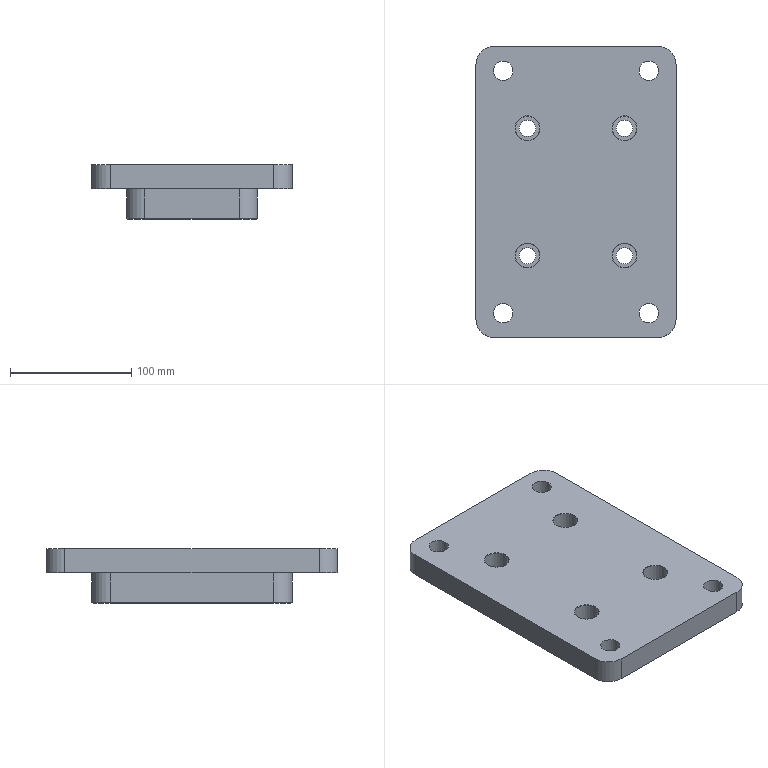NC program | NX | posted with a generic post | part box 165 x 240 x 45 mm
Lines 1 to 2077 of 2364, first 1783 of 2069 lines:
N10 G17 G21 G94 G90
(ZLEVEL_PROFILE_COPY , TOOL : D25R0.5)
N12 T05 M6
N14 G54
N16 G17 G0 G90 X-124.057 Y-0.073 S2000 M3
N18 G43 Z30. H5
N20 Z3.
N22 G94 G1 Y40.842 Z1.929 F1000.
N24 X-123.672 Y45.838 Z1.797
N26 X-122.847 Y50.78 Z1.666
N28 X-121.589 Y55.629 Z1.535
N30 X-119.906 Y60.348 Z1.404
N32 X-117.812 Y64.9 Z1.273
N34 X-115.324 Y69.249 Z1.141
N36 X-112.461 Y73.36 Z1.01
N38 X-109.245 Y77.203 Z0.879
N40 X-105.703 Y80.745 Z0.748
N42 X-101.86 Y83.961 Z0.617
N44 X-97.749 Y86.824 Z0.485
N46 X-93.4 Y89.312 Z0.354
N48 X-88.848 Y91.406 Z0.223
N50 X-84.129 Y93.089 Z0.092
N52 X-79.28 Y94.347 Z-0.039
N54 X-74.338 Y95.172 Z-0.171
N56 X-69.342 Y95.557 Z-0.302
N58 X-67.5 Z-0.35
N60 X67.5 F2200.
N62 G2 X124.057 Y39. R56.557
N64 G1 Y-39.
N66 G2 X67.5 Y-95.557 R56.557
N68 G1 X-67.5
N70 G2 X-124.057 Y-39. R56.557
N72 G1 Y39.
N74 G2 X-67.5 Y95.557 R56.557
N76 G1 X-47.449 Y95.907 Z-0.7
N78 X67.5
N80 G2 X124.407 Y39. R56.907
N82 G1 Y-39.
N84 G2 X67.5 Y-95.907 R56.907
N86 G1 X-67.5
N88 G2 X-124.407 Y-39. R56.907
N90 G1 Y39.
N92 G2 X-67.5 Y95.907 R56.907
N94 G1 X-47.449 Y96.257 Z-1.05
N96 X67.5
N98 G2 X124.757 Y39. R57.257
N100 G1 Y-39.
N102 G2 X67.5 Y-96.257 R57.257
N104 G1 X-67.5
N106 G2 X-124.757 Y-39. R57.257
N108 G1 Y39.
N110 G2 X-67.5 Y96.257 R57.257
N112 G1 X-63.044 Y96.335 Z-1.128
N114 X-61.93 Y96.354 Z-1.147
N116 X-60.816 Y96.373 Z-1.167
N118 X-59.702 Y96.389 Z-1.186
N120 X-58.588 Y96.404 Z-1.206
N122 X-57.474 Y96.418 Z-1.225
N124 X-56.36 Y96.43 Z-1.244
N126 X-55.246 Y96.441 Z-1.264
N128 X-54.132 Y96.451 Z-1.283
N130 X-53.018 Y96.459 Z-1.303
N132 X-51.904 Y96.467 Z-1.322
N134 X-50.79 Y96.474 Z-1.342
N136 X-49.676 Y96.48 Z-1.361
N138 X-48.562 Y96.486 Z-1.381
N140 X-47.449 Y96.49 Z-1.4
N142 X67.5
N144 G2 X124.99 Y39. R57.49
N146 G1 Y-39.
N148 G2 X67.5 Y-96.49 R57.49
N150 G1 X-67.5
N152 G2 X-124.99 Y-39. R57.49
N154 G1 Y39.
N156 G2 X-67.5 Y96.49 R57.49
N158 G1 X-66.386 Y96.493 Z-1.419
N160 X-65.272 Y96.496 Z-1.439
N162 X-64.158 Y96.498 Z-1.458
N164 X-63.044 Y96.5 Z-1.478
N166 X-61.93 Z-1.497
N168 X-60.816 Z-1.517
N170 X-47.449 Z-1.75
N172 X67.5
N174 G2 X125. Y39. R57.5
N176 G1 Y-39.
N178 G2 X67.5 Y-96.5 R57.5
N180 G1 X-67.5
N182 G2 X-125. Y-39. R57.5
N184 G1 Y39.
N186 G2 X-67.5 Y96.5 R57.5
N188 G1 X-47.449 Z-2.1
N190 X67.5
N192 G2 X125. Y39. R57.5
N194 G1 Y-39.
N196 G2 X67.5 Y-96.5 R57.5
N198 G1 X-67.5
N200 G2 X-125. Y-39. R57.5
N202 G1 Y39.
N204 G2 X-67.5 Y96.5 R57.5
N206 G1 X-47.449 Z-2.45
N208 X67.5
N210 G2 X125. Y39. R57.5
N212 G1 Y-39.
N214 G2 X67.5 Y-96.5 R57.5
N216 G1 X-67.5
N218 G2 X-125. Y-39. R57.5
N220 G1 Y39.
N222 G2 X-67.5 Y96.5 R57.5
N224 G1 X-47.449 Z-2.8
N226 X67.5
N228 G2 X125. Y39. R57.5
N230 G1 Y-39.
N232 G2 X67.5 Y-96.5 R57.5
N234 G1 X-67.5
N236 G2 X-125. Y-39. R57.5
N238 G1 Y39.
N240 G2 X-67.5 Y96.5 R57.5
N242 G1 X-47.449 Z-3.15
N244 X67.5
N246 G2 X125. Y39. R57.5
N248 G1 Y-39.
N250 G2 X67.5 Y-96.5 R57.5
N252 G1 X-67.5
N254 G2 X-125. Y-39. R57.5
N256 G1 Y39.
N258 G2 X-67.5 Y96.5 R57.5
N260 G1 X-47.449 Z-3.5
N262 X67.5
N264 G2 X125. Y39. R57.5
N266 G1 Y-39.
N268 G2 X67.5 Y-96.5 R57.5
N270 G1 X-67.5
N272 G2 X-125. Y-39. R57.5
N274 G1 Y39.
N276 G2 X-67.5 Y96.5 R57.5
N278 G1 X-47.449 Z-3.85
N280 X67.5
N282 G2 X125. Y39. R57.5
N284 G1 Y-39.
N286 G2 X67.5 Y-96.5 R57.5
N288 G1 X-67.5
N290 G2 X-125. Y-39. R57.5
N292 G1 Y39.
N294 G2 X-67.5 Y96.5 R57.5
N296 G1 X-47.449 Z-4.2
N298 X67.5
N300 G2 X125. Y39. R57.5
N302 G1 Y-39.
N304 G2 X67.5 Y-96.5 R57.5
N306 G1 X-67.5
N308 G2 X-125. Y-39. R57.5
N310 G1 Y39.
N312 G2 X-67.5 Y96.5 R57.5
N314 G1 X-47.449 Z-4.55
N316 X67.5
N318 G2 X125. Y39. R57.5
N320 G1 Y-39.
N322 G2 X67.5 Y-96.5 R57.5
N324 G1 X-67.5
N326 G2 X-125. Y-39. R57.5
N328 G1 Y39.
N330 G2 X-67.5 Y96.5 R57.5
N332 G1 X-47.449 Z-4.9
N334 X67.5
N336 G2 X125. Y39. R57.5
N338 G1 Y-39.
N340 G2 X67.5 Y-96.5 R57.5
N342 G1 X-67.5
N344 G2 X-125. Y-39. R57.5
N346 G1 Y39.
N348 G2 X-67.5 Y96.5 R57.5
N350 G1 X-47.449 Z-5.25
N352 X67.5
N354 G2 X125. Y39. R57.5
N356 G1 Y-39.
N358 G2 X67.5 Y-96.5 R57.5
N360 G1 X-67.5
N362 G2 X-125. Y-39. R57.5
N364 G1 Y39.
N366 G2 X-67.5 Y96.5 R57.5
N368 G1 X-47.449 Z-5.6
N370 X67.5
N372 G2 X125. Y39. R57.5
N374 G1 Y-39.
N376 G2 X67.5 Y-96.5 R57.5
N378 G1 X-67.5
N380 G2 X-125. Y-39. R57.5
N382 G1 Y39.
N384 G2 X-67.5 Y96.5 R57.5
N386 G1 X-47.449 Z-5.95
N388 X67.5
N390 G2 X125. Y39. R57.5
N392 G1 Y-39.
N394 G2 X67.5 Y-96.5 R57.5
N396 G1 X-67.5
N398 G2 X-125. Y-39. R57.5
N400 G1 Y39.
N402 G2 X-67.5 Y96.5 R57.5
N404 G1 X-47.449 Z-6.3
N406 X67.5
N408 G2 X125. Y39. R57.5
N410 G1 Y-39.
N412 G2 X67.5 Y-96.5 R57.5
N414 G1 X-67.5
N416 G2 X-125. Y-39. R57.5
N418 G1 Y39.
N420 G2 X-67.5 Y96.5 R57.5
N422 G1 X-47.449 Z-6.65
N424 X67.5
N426 G2 X125. Y39. R57.5
N428 G1 Y-39.
N430 G2 X67.5 Y-96.5 R57.5
N432 G1 X-67.5
N434 G2 X-125. Y-39. R57.5
N436 G1 Y39.
N438 G2 X-67.5 Y96.5 R57.5
N440 G1 X-47.449 Z-7.
N442 X67.5
N444 G2 X125. Y39. R57.5
N446 G1 Y-39.
N448 G2 X67.5 Y-96.5 R57.5
N450 G1 X-67.5
N452 G2 X-125. Y-39. R57.5
N454 G1 Y39.
N456 G2 X-67.5 Y96.5 R57.5
N458 G1 X-47.449 Z-7.35
N460 X67.5
N462 G2 X125. Y39. R57.5
N464 G1 Y-39.
N466 G2 X67.5 Y-96.5 R57.5
N468 G1 X-67.5
N470 G2 X-125. Y-39. R57.5
N472 G1 Y39.
N474 G2 X-67.5 Y96.5 R57.5
N476 G1 X-47.449 Z-7.7
N478 X67.5
N480 G2 X125. Y39. R57.5
N482 G1 Y-39.
N484 G2 X67.5 Y-96.5 R57.5
N486 G1 X-67.5
N488 G2 X-125. Y-39. R57.5
N490 G1 Y39.
N492 G2 X-67.5 Y96.5 R57.5
N494 G1 X-47.449 Z-8.05
N496 X67.5
N498 G2 X125. Y39. R57.5
N500 G1 Y-39.
N502 G2 X67.5 Y-96.5 R57.5
N504 G1 X-67.5
N506 G2 X-125. Y-39. R57.5
N508 G1 Y39.
N510 G2 X-67.5 Y96.5 R57.5
N512 G1 X-47.449 Z-8.4
N514 X67.5
N516 G2 X125. Y39. R57.5
N518 G1 Y-39.
N520 G2 X67.5 Y-96.5 R57.5
N522 G1 X-67.5
N524 G2 X-125. Y-39. R57.5
N526 G1 Y39.
N528 G2 X-67.5 Y96.5 R57.5
N530 G1 X-47.449 Z-8.75
N532 X67.5
N534 G2 X125. Y39. R57.5
N536 G1 Y-39.
N538 G2 X67.5 Y-96.5 R57.5
N540 G1 X-67.5
N542 G2 X-125. Y-39. R57.5
N544 G1 Y39.
N546 G2 X-67.5 Y96.5 R57.5
N548 G1 X-47.449 Z-9.1
N550 X67.5
N552 G2 X125. Y39. R57.5
N554 G1 Y-39.
N556 G2 X67.5 Y-96.5 R57.5
N558 G1 X-67.5
N560 G2 X-125. Y-39. R57.5
N562 G1 Y39.
N564 G2 X-67.5 Y96.5 R57.5
N566 G1 X-47.449 Z-9.45
N568 X67.5
N570 G2 X125. Y39. R57.5
N572 G1 Y-39.
N574 G2 X67.5 Y-96.5 R57.5
N576 G1 X-67.5
N578 G2 X-125. Y-39. R57.5
N580 G1 Y39.
N582 G2 X-67.5 Y96.5 R57.5
N584 G1 X-47.449 Z-9.8
N586 X67.5
N588 G2 X125. Y39. R57.5
N590 G1 Y-39.
N592 G2 X67.5 Y-96.5 R57.5
N594 G1 X-67.5
N596 G2 X-125. Y-39. R57.5
N598 G1 Y39.
N600 G2 X-67.5 Y96.5 R57.5
N602 G1 X-47.449 Z-10.15
N604 X67.5
N606 G2 X125. Y39. R57.5
N608 G1 Y-39.
N610 G2 X67.5 Y-96.5 R57.5
N612 G1 X-67.5
N614 G2 X-125. Y-39. R57.5
N616 G1 Y39.
N618 G2 X-67.5 Y96.5 R57.5
N620 G1 X-47.449 Z-10.5
N622 X67.5
N624 G2 X125. Y39. R57.5
N626 G1 Y-39.
N628 G2 X67.5 Y-96.5 R57.5
N630 G1 X-67.5
N632 G2 X-125. Y-39. R57.5
N634 G1 Y39.
N636 G2 X-67.5 Y96.5 R57.5
N638 G1 X-47.449 Z-10.85
N640 X67.5
N642 G2 X125. Y39. R57.5
N644 G1 Y-39.
N646 G2 X67.5 Y-96.5 R57.5
N648 G1 X-67.5
N650 G2 X-125. Y-39. R57.5
N652 G1 Y39.
N654 G2 X-67.5 Y96.5 R57.5
N656 G1 X-47.449 Z-11.2
N658 X67.5
N660 G2 X125. Y39. R57.5
N662 G1 Y-39.
N664 G2 X67.5 Y-96.5 R57.5
N666 G1 X-67.5
N668 G2 X-125. Y-39. R57.5
N670 G1 Y39.
N672 G2 X-67.5 Y96.5 R57.5
N674 G1 X-47.449 Z-11.55
N676 X67.5
N678 G2 X125. Y39. R57.5
N680 G1 Y-39.
N682 G2 X67.5 Y-96.5 R57.5
N684 G1 X-67.5
N686 G2 X-125. Y-39. R57.5
N688 G1 Y39.
N690 G2 X-67.5 Y96.5 R57.5
N692 G1 X-47.449 Z-11.9
N694 X67.5
N696 G2 X125. Y39. R57.5
N698 G1 Y-39.
N700 G2 X67.5 Y-96.5 R57.5
N702 G1 X-67.5
N704 G2 X-125. Y-39. R57.5
N706 G1 Y39.
N708 G2 X-67.5 Y96.5 R57.5
N710 G1 X-47.449 Z-12.25
N712 X67.5
N714 G2 X125. Y39. R57.5
N716 G1 Y-39.
N718 G2 X67.5 Y-96.5 R57.5
N720 G1 X-67.5
N722 G2 X-125. Y-39. R57.5
N724 G1 Y39.
N726 G2 X-67.5 Y96.5 R57.5
N728 G1 X-47.449 Z-12.6
N730 X67.5
N732 G2 X125. Y39. R57.5
N734 G1 Y-39.
N736 G2 X67.5 Y-96.5 R57.5
N738 G1 X-67.5
N740 G2 X-125. Y-39. R57.5
N742 G1 Y39.
N744 G2 X-67.5 Y96.5 R57.5
N746 G1 X-47.449 Z-12.95
N748 X67.5
N750 G2 X125. Y39. R57.5
N752 G1 Y-39.
N754 G2 X67.5 Y-96.5 R57.5
N756 G1 X-67.5
N758 G2 X-125. Y-39. R57.5
N760 G1 Y39.
N762 G2 X-67.5 Y96.5 R57.5
N764 G1 X-47.449 Z-13.3
N766 X67.5
N768 G2 X125. Y39. R57.5
N770 G1 Y-39.
N772 G2 X67.5 Y-96.5 R57.5
N774 G1 X-67.5
N776 G2 X-125. Y-39. R57.5
N778 G1 Y39.
N780 G2 X-67.5 Y96.5 R57.5
N782 G1 X-47.449 Z-13.65
N784 X67.5
N786 G2 X125. Y39. R57.5
N788 G1 Y-39.
N790 G2 X67.5 Y-96.5 R57.5
N792 G1 X-67.5
N794 G2 X-125. Y-39. R57.5
N796 G1 Y39.
N798 G2 X-67.5 Y96.5 R57.5
N800 G1 X-47.449 Z-14.
N802 X67.5
N804 G2 X125. Y39. R57.5
N806 G1 Y-39.
N808 G2 X67.5 Y-96.5 R57.5
N810 G1 X-67.5
N812 G2 X-125. Y-39. R57.5
N814 G1 Y39.
N816 G2 X-67.5 Y96.5 R57.5
N818 G1 X-47.449 Z-14.35
N820 X67.5
N822 G2 X125. Y39. R57.5
N824 G1 Y-39.
N826 G2 X67.5 Y-96.5 R57.5
N828 G1 X-67.5
N830 G2 X-125. Y-39. R57.5
N832 G1 Y39.
N834 G2 X-67.5 Y96.5 R57.5
N836 G1 X-47.449 Z-14.7
N838 X67.5
N840 G2 X125. Y39. R57.5
N842 G1 Y-39.
N844 G2 X67.5 Y-96.5 R57.5
N846 G1 X-67.5
N848 G2 X-125. Y-39. R57.5
N850 G1 Y39.
N852 G2 X-67.5 Y96.5 R57.5
N854 G1 X-47.449 Z-15.05
N856 X67.5
N858 G2 X125. Y39. R57.5
N860 G1 Y-39.
N862 G2 X67.5 Y-96.5 R57.5
N864 G1 X-67.5
N866 G2 X-125. Y-39. R57.5
N868 G1 Y39.
N870 G2 X-67.5 Y96.5 R57.5
N872 G1 X-47.449 Z-15.4
N874 X67.5
N876 G2 X125. Y39. R57.5
N878 G1 Y-39.
N880 G2 X67.5 Y-96.5 R57.5
N882 G1 X-67.5
N884 G2 X-125. Y-39. R57.5
N886 G1 Y39.
N888 G2 X-67.5 Y96.5 R57.5
N890 G1 X-47.449 Z-15.75
N892 X67.5
N894 G2 X125. Y39. R57.5
N896 G1 Y-39.
N898 G2 X67.5 Y-96.5 R57.5
N900 G1 X-67.5
N902 G2 X-125. Y-39. R57.5
N904 G1 Y39.
N906 G2 X-67.5 Y96.5 R57.5
N908 G1 X-47.449 Z-16.1
N910 X67.5
N912 G2 X125. Y39. R57.5
N914 G1 Y-39.
N916 G2 X67.5 Y-96.5 R57.5
N918 G1 X-67.5
N920 G2 X-125. Y-39. R57.5
N922 G1 Y39.
N924 G2 X-67.5 Y96.5 R57.5
N926 G1 X-47.449 Z-16.45
N928 X67.5
N930 G2 X125. Y39. R57.5
N932 G1 Y-39.
N934 G2 X67.5 Y-96.5 R57.5
N936 G1 X-67.5
N938 G2 X-125. Y-39. R57.5
N940 G1 Y39.
N942 G2 X-67.5 Y96.5 R57.5
N944 G1 X-47.449 Z-16.8
N946 X67.5
N948 G2 X125. Y39. R57.5
N950 G1 Y-39.
N952 G2 X67.5 Y-96.5 R57.5
N954 G1 X-67.5
N956 G2 X-125. Y-39. R57.5
N958 G1 Y39.
N960 G2 X-67.5 Y96.5 R57.5
N962 G1 X-47.449 Z-17.15
N964 X67.5
N966 G2 X125. Y39. R57.5
N968 G1 Y-39.
N970 G2 X67.5 Y-96.5 R57.5
N972 G1 X-67.5
N974 G2 X-125. Y-39. R57.5
N976 G1 Y39.
N978 G2 X-67.5 Y96.5 R57.5
N980 G1 X-47.449 Z-17.5
N982 X67.5
N984 G2 X125. Y39. R57.5
N986 G1 Y-39.
N988 G2 X67.5 Y-96.5 R57.5
N990 G1 X-67.5
N992 G2 X-125. Y-39. R57.5
N994 G1 Y39.
N996 G2 X-67.5 Y96.5 R57.5
N998 G1 X-47.449 Z-17.85
N1000 X67.5
N1002 G2 X125. Y39. R57.5
N1004 G1 Y-39.
N1006 G2 X67.5 Y-96.5 R57.5
N1008 G1 X-67.5
N1010 G2 X-125. Y-39. R57.5
N1012 G1 Y39.
N1014 G2 X-67.5 Y96.5 R57.5
N1016 G1 X-47.449 Z-18.2
N1018 X67.5
N1020 G2 X125. Y39. R57.5
N1022 G1 Y-39.
N1024 G2 X67.5 Y-96.5 R57.5
N1026 G1 X-67.5
N1028 G2 X-125. Y-39. R57.5
N1030 G1 Y39.
N1032 G2 X-67.5 Y96.5 R57.5
N1034 G1 X-47.449 Z-18.55
N1036 X67.5
N1038 G2 X125. Y39. R57.5
N1040 G1 Y-39.
N1042 G2 X67.5 Y-96.5 R57.5
N1044 G1 X-67.5
N1046 G2 X-125. Y-39. R57.5
N1048 G1 Y39.
N1050 G2 X-67.5 Y96.5 R57.5
N1052 G1 X-47.449 Z-18.9
N1054 X67.5
N1056 G2 X125. Y39. R57.5
N1058 G1 Y-39.
N1060 G2 X67.5 Y-96.5 R57.5
N1062 G1 X-67.5
N1064 G2 X-125. Y-39. R57.5
N1066 G1 Y39.
N1068 G2 X-67.5 Y96.5 R57.5
N1070 G1 X-47.449 Z-19.25
N1072 X67.5
N1074 G2 X125. Y39. R57.5
N1076 G1 Y-39.
N1078 G2 X67.5 Y-96.5 R57.5
N1080 G1 X-67.5
N1082 G2 X-125. Y-39. R57.5
N1084 G1 Y39.
N1086 G2 X-67.5 Y96.5 R57.5
N1088 G1 X-47.449 Z-19.6
N1090 X67.5
N1092 G2 X125. Y39. R57.5
N1094 G1 Y-39.
N1096 G2 X67.5 Y-96.5 R57.5
N1098 G1 X-67.5
N1100 G2 X-125. Y-39. R57.5
N1102 G1 Y39.
N1104 G2 X-67.5 Y96.5 R57.5
N1106 G1 X-47.449 Z-19.95
N1108 X67.5
N1110 G2 X125. Y39. R57.5
N1112 G1 Y-39.
N1114 G2 X67.5 Y-96.5 R57.5
N1116 G1 X-67.5
N1118 G2 X-125. Y-39. R57.5
N1120 G1 Y39.
N1122 G2 X-67.5 Y96.5 R57.5
N1124 G1 X-47.449 Z-20.3
N1126 X67.5
N1128 G2 X125. Y39. R57.5
N1130 G1 Y-39.
N1132 G2 X67.5 Y-96.5 R57.5
N1134 G1 X-67.5
N1136 G2 X-125. Y-39. R57.5
N1138 G1 Y39.
N1140 G2 X-67.5 Y96.5 R57.5
N1142 G1 X-47.449 Z-20.65
N1144 X67.5
N1146 G2 X125. Y39. R57.5
N1148 G1 Y-39.
N1150 G2 X67.5 Y-96.5 R57.5
N1152 G1 X-67.5
N1154 G2 X-125. Y-39. R57.5
N1156 G1 Y39.
N1158 G2 X-67.5 Y96.5 R57.5
N1160 G1 X-47.449 Z-21.
N1162 X67.5
N1164 G2 X125. Y39. R57.5
N1166 G1 Y-39.
N1168 G2 X67.5 Y-96.5 R57.5
N1170 G1 X-67.5
N1172 G2 X-125. Y-39. R57.5
N1174 G1 Y39.
N1176 G2 X-67.5 Y96.5 R57.5
N1178 G1 X-47.449 Z-21.35
N1180 X67.5
N1182 G2 X125. Y39. R57.5
N1184 G1 Y-39.
N1186 G2 X67.5 Y-96.5 R57.5
N1188 G1 X-67.5
N1190 G2 X-125. Y-39. R57.5
N1192 G1 Y39.
N1194 G2 X-67.5 Y96.5 R57.5
N1196 G1 X-47.449 Z-21.7
N1198 X67.5
N1200 G2 X125. Y39. R57.5
N1202 G1 Y-39.
N1204 G2 X67.5 Y-96.5 R57.5
N1206 G1 X-67.5
N1208 G2 X-125. Y-39. R57.5
N1210 G1 Y39.
N1212 G2 X-67.5 Y96.5 R57.5
N1214 G1 X-47.449 Z-22.05
N1216 X67.5
N1218 G2 X125. Y39. R57.5
N1220 G1 Y-39.
N1222 G2 X67.5 Y-96.5 R57.5
N1224 G1 X-67.5
N1226 G2 X-125. Y-39. R57.5
N1228 G1 Y39.
N1230 G2 X-67.5 Y96.5 R57.5
N1232 G1 X-47.449 Z-22.4
N1234 X67.5
N1236 G2 X125. Y39. R57.5
N1238 G1 Y-39.
N1240 G2 X67.5 Y-96.5 R57.5
N1242 G1 X-67.5
N1244 G2 X-125. Y-39. R57.5
N1246 G1 Y39.
N1248 G2 X-67.5 Y96.5 R57.5
N1250 G1 X-47.449 Z-22.75
N1252 X67.5
N1254 G2 X125. Y39. R57.5
N1256 G1 Y-39.
N1258 G2 X67.5 Y-96.5 R57.5
N1260 G1 X-67.5
N1262 G2 X-125. Y-39. R57.5
N1264 G1 Y39.
N1266 G2 X-67.5 Y96.5 R57.5
N1268 G1 X-47.449 Z-23.1
N1270 X67.5
N1272 G2 X125. Y39. R57.5
N1274 G1 Y-39.
N1276 G2 X67.5 Y-96.5 R57.5
N1278 G1 X-67.5
N1280 G2 X-125. Y-39. R57.5
N1282 G1 Y39.
N1284 G2 X-67.5 Y96.5 R57.5
N1286 G1 X-47.449 Z-23.45
N1288 X67.5
N1290 G2 X125. Y39. R57.5
N1292 G1 Y-39.
N1294 G2 X67.5 Y-96.5 R57.5
N1296 G1 X-67.5
N1298 G2 X-125. Y-39. R57.5
N1300 G1 Y39.
N1302 G2 X-67.5 Y96.5 R57.5
N1304 G1 X-47.449 Z-23.8
N1306 X67.5
N1308 G2 X125. Y39. R57.5
N1310 G1 Y-39.
N1312 G2 X67.5 Y-96.5 R57.5
N1314 G1 X-67.5
N1316 G2 X-125. Y-39. R57.5
N1318 G1 Y39.
N1320 G2 X-67.5 Y96.5 R57.5
N1322 G1 X-47.449 Z-24.15
N1324 X67.5
N1326 G2 X125. Y39. R57.5
N1328 G1 Y-39.
N1330 G2 X67.5 Y-96.5 R57.5
N1332 G1 X-67.5
N1334 G2 X-125. Y-39. R57.5
N1336 G1 Y39.
N1338 G2 X-67.5 Y96.5 R57.5
N1340 G1 X-47.449 Z-24.5
N1342 X67.5
N1344 G2 X125. Y39. R57.5
N1346 G1 Y-39.
N1348 G2 X67.5 Y-96.5 R57.5
N1350 G1 X-67.5
N1352 G2 X-125. Y-39. R57.5
N1354 G1 Y39.
N1356 G2 X-67.5 Y96.5 R57.5
N1358 G1 X-47.449 Z-24.85
N1360 X67.5
N1362 G2 X125. Y39. R57.5
N1364 G1 Y-39.
N1366 G2 X67.5 Y-96.5 R57.5
N1368 G1 X-67.5
N1370 G2 X-125. Y-39. R57.5
N1372 G1 Y39.
N1374 G2 X-67.5 Y96.5 R57.5
N1376 G1 X-47.449
N1378 Z-21.85
N1380 G0 Z30.
(ZLEVEL_PROFILE_COPY_COPY_COPY , TOOL : D25R0.5)
N1382 X-109.057 Y-23.637
N1384 Z3.
N1386 G1 Y40.579 Z1.318 F1000.
N1388 X-108.652 Y44.999 Z1.202
N1390 X-107.778 Y49.351 Z1.086
N1392 X-106.446 Y53.584 Z0.97
N1394 X-104.67 Y57.652 Z0.854
N1396 X-102.471 Y61.507 Z0.737
N1398 X-99.873 Y65.105 Z0.621
N1400 X-96.907 Y68.407 Z0.505
N1402 X-93.605 Y71.373 Z0.389
N1404 X-90.007 Y73.971 Z0.272
N1406 X-86.152 Y76.17 Z0.156
N1408 X-82.084 Y77.946 Z0.04
N1410 X-77.851 Y79.278 Z-0.076
N1412 X-73.499 Y80.152 Z-0.192
N1414 X-69.079 Y80.557 Z-0.309
N1416 X-67.5 Z-0.35
N1418 X67.5 F2200.
N1420 G2 X109.057 Y39. R41.557
N1422 G1 Y-39.
N1424 G2 X67.5 Y-80.557 R41.557
N1426 G1 X-67.5
N1428 G2 X-109.057 Y-39. R41.557
N1430 G1 Y39.
N1432 G2 X-67.5 Y80.557 R41.557
N1434 G1 X-47.449 Y80.907 Z-0.7
N1436 X67.5
N1438 G2 X109.407 Y39. R41.907
N1440 G1 Y-39.
N1442 G2 X67.5 Y-80.907 R41.907
N1444 G1 X-67.5
N1446 G2 X-109.407 Y-39. R41.907
N1448 G1 Y39.
N1450 G2 X-67.5 Y80.907 R41.907
N1452 G1 X-47.449 Y81.257 Z-1.05
N1454 X67.5
N1456 G2 X109.757 Y39. R42.257
N1458 G1 Y-39.
N1460 G2 X67.5 Y-81.257 R42.257
N1462 G1 X-67.5
N1464 G2 X-109.757 Y-39. R42.257
N1466 G1 Y39.
N1468 G2 X-67.5 Y81.257 R42.257
N1470 G1 X-62.487 Y81.345 Z-1.138
N1472 X-61.652 Y81.359 Z-1.152
N1474 X-60.816 Y81.373 Z-1.167
N1476 X-59.981 Y81.385 Z-1.181
N1478 X-59.145 Y81.397 Z-1.196
N1480 X-58.31 Y81.408 Z-1.21
N1482 X-57.474 Y81.418 Z-1.225
N1484 X-56.639 Y81.427 Z-1.24
N1486 X-55.803 Y81.435 Z-1.254
N1488 X-54.968 Y81.443 Z-1.269
N1490 X-54.132 Y81.451 Z-1.283
N1492 X-53.297 Y81.457 Z-1.298
N1494 X-52.461 Y81.464 Z-1.313
N1496 X-51.626 Y81.469 Z-1.327
N1498 X-50.79 Y81.474 Z-1.342
N1500 X-49.955 Y81.479 Z-1.356
N1502 X-49.119 Y81.483 Z-1.371
N1504 X-48.284 Y81.487 Z-1.385
N1506 X-47.449 Y81.49 Z-1.4
N1508 X67.5
N1510 G2 X109.99 Y39. R42.49
N1512 G1 Y-39.
N1514 G2 X67.5 Y-81.49 R42.49
N1516 G1 X-67.5
N1518 G2 X-109.99 Y-39. R42.49
N1520 G1 Y39.
N1522 G2 X-67.5 Y81.49 R42.49
N1524 G1 X-66.665 Y81.493 Z-1.415
N1526 X-65.829 Y81.495 Z-1.429
N1528 X-64.994 Y81.497 Z-1.444
N1530 X-64.158 Y81.498 Z-1.458
N1532 X-63.323 Y81.499 Z-1.473
N1534 X-62.487 Y81.5 Z-1.488
N1536 X-61.652 Z-1.502
N1538 X-47.449 Z-1.75
N1540 X67.5
N1542 G2 X110. Y39. R42.5
N1544 G1 Y-39.
N1546 G2 X67.5 Y-81.5 R42.5
N1548 G1 X-67.5
N1550 G2 X-110. Y-39. R42.5
N1552 G1 Y39.
N1554 G2 X-67.5 Y81.5 R42.5
N1556 G1 X-47.449 Z-2.1
N1558 X67.5
N1560 G2 X110. Y39. R42.5
N1562 G1 Y-39.
N1564 G2 X67.5 Y-81.5 R42.5
N1566 G1 X-67.5
N1568 G2 X-110. Y-39. R42.5
N1570 G1 Y39.
N1572 G2 X-67.5 Y81.5 R42.5
N1574 G1 X-47.449 Z-2.45
N1576 X67.5
N1578 G2 X110. Y39. R42.5
N1580 G1 Y-39.
N1582 G2 X67.5 Y-81.5 R42.5
N1584 G1 X-67.5
N1586 G2 X-110. Y-39. R42.5
N1588 G1 Y39.
N1590 G2 X-67.5 Y81.5 R42.5
N1592 G1 X-47.449 Z-2.8
N1594 X67.5
N1596 G2 X110. Y39. R42.5
N1598 G1 Y-39.
N1600 G2 X67.5 Y-81.5 R42.5
N1602 G1 X-67.5
N1604 G2 X-110. Y-39. R42.5
N1606 G1 Y39.
N1608 G2 X-67.5 Y81.5 R42.5
N1610 G1 X-47.449 Z-3.15
N1612 X67.5
N1614 G2 X110. Y39. R42.5
N1616 G1 Y-39.
N1618 G2 X67.5 Y-81.5 R42.5
N1620 G1 X-67.5
N1622 G2 X-110. Y-39. R42.5
N1624 G1 Y39.
N1626 G2 X-67.5 Y81.5 R42.5
N1628 G1 X-47.449 Z-3.5
N1630 X67.5
N1632 G2 X110. Y39. R42.5
N1634 G1 Y-39.
N1636 G2 X67.5 Y-81.5 R42.5
N1638 G1 X-67.5
N1640 G2 X-110. Y-39. R42.5
N1642 G1 Y39.
N1644 G2 X-67.5 Y81.5 R42.5
N1646 G1 X-47.449 Z-3.85
N1648 X67.5
N1650 G2 X110. Y39. R42.5
N1652 G1 Y-39.
N1654 G2 X67.5 Y-81.5 R42.5
N1656 G1 X-67.5
N1658 G2 X-110. Y-39. R42.5
N1660 G1 Y39.
N1662 G2 X-67.5 Y81.5 R42.5
N1664 G1 X-47.449 Z-4.2
N1666 X67.5
N1668 G2 X110. Y39. R42.5
N1670 G1 Y-39.
N1672 G2 X67.5 Y-81.5 R42.5
N1674 G1 X-67.5
N1676 G2 X-110. Y-39. R42.5
N1678 G1 Y39.
N1680 G2 X-67.5 Y81.5 R42.5
N1682 G1 X-47.449 Z-4.55
N1684 X67.5
N1686 G2 X110. Y39. R42.5
N1688 G1 Y-39.
N1690 G2 X67.5 Y-81.5 R42.5
N1692 G1 X-67.5
N1694 G2 X-110. Y-39. R42.5
N1696 G1 Y39.
N1698 G2 X-67.5 Y81.5 R42.5
N1700 G1 X-47.449 Z-4.9
N1702 X67.5
N1704 G2 X110. Y39. R42.5
N1706 G1 Y-39.
N1708 G2 X67.5 Y-81.5 R42.5
N1710 G1 X-67.5
N1712 G2 X-110. Y-39. R42.5
N1714 G1 Y39.
N1716 G2 X-67.5 Y81.5 R42.5
N1718 G1 X-47.449 Z-5.25
N1720 X67.5
N1722 G2 X110. Y39. R42.5
N1724 G1 Y-39.
N1726 G2 X67.5 Y-81.5 R42.5
N1728 G1 X-67.5
N1730 G2 X-110. Y-39. R42.5
N1732 G1 Y39.
N1734 G2 X-67.5 Y81.5 R42.5
N1736 G1 X-47.449 Z-5.6
N1738 X67.5
N1740 G2 X110. Y39. R42.5
N1742 G1 Y-39.
N1744 G2 X67.5 Y-81.5 R42.5
N1746 G1 X-67.5
N1748 G2 X-110. Y-39. R42.5
N1750 G1 Y39.
N1752 G2 X-67.5 Y81.5 R42.5
N1754 G1 X-47.449 Z-5.95
N1756 X67.5
N1758 G2 X110. Y39. R42.5
N1760 G1 Y-39.
N1762 G2 X67.5 Y-81.5 R42.5
N1764 G1 X-67.5
N1766 G2 X-110. Y-39. R42.5
N1768 G1 Y39.
N1770 G2 X-67.5 Y81.5 R42.5
N1772 G1 X-47.449 Z-6.3
N1774 X67.5
N1776 G2 X110. Y39. R42.5
N1778 G1 Y-39.
N1780 G2 X67.5 Y-81.5 R42.5
N1782 G1 X-67.5
N1784 G2 X-110. Y-39. R42.5
N1786 G1 Y39.
N1788 G2 X-67.5 Y81.5 R42.5
N1790 G1 X-47.449 Z-6.65
N1792 X67.5
N1794 G2 X110. Y39. R42.5
N1796 G1 Y-39.
N1798 G2 X67.5 Y-81.5 R42.5
N1800 G1 X-67.5
N1802 G2 X-110. Y-39. R42.5
N1804 G1 Y39.
N1806 G2 X-67.5 Y81.5 R42.5
N1808 G1 X-47.449 Z-7.
N1810 X67.5
N1812 G2 X110. Y39. R42.5
N1814 G1 Y-39.
N1816 G2 X67.5 Y-81.5 R42.5
N1818 G1 X-67.5
N1820 G2 X-110. Y-39. R42.5
N1822 G1 Y39.
N1824 G2 X-67.5 Y81.5 R42.5
N1826 G1 X-47.449 Z-7.35
N1828 X67.5
N1830 G2 X110. Y39. R42.5
N1832 G1 Y-39.
N1834 G2 X67.5 Y-81.5 R42.5
N1836 G1 X-67.5
N1838 G2 X-110. Y-39. R42.5
N1840 G1 Y39.
N1842 G2 X-67.5 Y81.5 R42.5
N1844 G1 X-47.449 Z-7.7
N1846 X67.5
N1848 G2 X110. Y39. R42.5
N1850 G1 Y-39.
N1852 G2 X67.5 Y-81.5 R42.5
N1854 G1 X-67.5
N1856 G2 X-110. Y-39. R42.5
N1858 G1 Y39.
N1860 G2 X-67.5 Y81.5 R42.5
N1862 G1 X-47.449 Z-8.05
N1864 X67.5
N1866 G2 X110. Y39. R42.5
N1868 G1 Y-39.
N1870 G2 X67.5 Y-81.5 R42.5
N1872 G1 X-67.5
N1874 G2 X-110. Y-39. R42.5
N1876 G1 Y39.
N1878 G2 X-67.5 Y81.5 R42.5
N1880 G1 X-47.449 Z-8.4
N1882 X67.5
N1884 G2 X110. Y39. R42.5
N1886 G1 Y-39.
N1888 G2 X67.5 Y-81.5 R42.5
N1890 G1 X-67.5
N1892 G2 X-110. Y-39. R42.5
N1894 G1 Y39.
N1896 G2 X-67.5 Y81.5 R42.5
N1898 G1 X-47.449 Z-8.75
N1900 X67.5
N1902 G2 X110. Y39. R42.5
N1904 G1 Y-39.
N1906 G2 X67.5 Y-81.5 R42.5
N1908 G1 X-67.5
N1910 G2 X-110. Y-39. R42.5
N1912 G1 Y39.
N1914 G2 X-67.5 Y81.5 R42.5
N1916 G1 X-47.449 Z-9.1
N1918 X67.5
N1920 G2 X110. Y39. R42.5
N1922 G1 Y-39.
N1924 G2 X67.5 Y-81.5 R42.5
N1926 G1 X-67.5
N1928 G2 X-110. Y-39. R42.5
N1930 G1 Y39.
N1932 G2 X-67.5 Y81.5 R42.5
N1934 G1 X-47.449 Z-9.45
N1936 X67.5
N1938 G2 X110. Y39. R42.5
N1940 G1 Y-39.
N1942 G2 X67.5 Y-81.5 R42.5
N1944 G1 X-67.5
N1946 G2 X-110. Y-39. R42.5
N1948 G1 Y39.
N1950 G2 X-67.5 Y81.5 R42.5
N1952 G1 X-47.449 Z-9.8
N1954 X67.5
N1956 G2 X110. Y39. R42.5
N1958 G1 Y-39.
N1960 G2 X67.5 Y-81.5 R42.5
N1962 G1 X-67.5
N1964 G2 X-110. Y-39. R42.5
N1966 G1 Y39.
N1968 G2 X-67.5 Y81.5 R42.5
N1970 G1 X-47.449 Z-10.15
N1972 X67.5
N1974 G2 X110. Y39. R42.5
N1976 G1 Y-39.
N1978 G2 X67.5 Y-81.5 R42.5
N1980 G1 X-67.5
N1982 G2 X-110. Y-39. R42.5
N1984 G1 Y39.
N1986 G2 X-67.5 Y81.5 R42.5
N1988 G1 X-47.449 Z-10.5
N1990 X67.5
N1992 G2 X110. Y39. R42.5
N1994 G1 Y-39.
N1996 G2 X67.5 Y-81.5 R42.5
N1998 G1 X-67.5
N2000 G2 X-110. Y-39. R42.5
N2002 G1 Y39.
N2004 G2 X-67.5 Y81.5 R42.5
N2006 G1 X-47.449 Z-10.85
N2008 X67.5
N2010 G2 X110. Y39. R42.5
N2012 G1 Y-39.
N2014 G2 X67.5 Y-81.5 R42.5
N2016 G1 X-67.5
N2018 G2 X-110. Y-39. R42.5
N2020 G1 Y39.
N2022 G2 X-67.5 Y81.5 R42.5
N2024 G1 X-47.449 Z-11.2
N2026 X67.5
N2028 G2 X110. Y39. R42.5
N2030 G1 Y-39.
N2032 G2 X67.5 Y-81.5 R42.5
N2034 G1 X-67.5
N2036 G2 X-110. Y-39. R42.5
N2038 G1 Y39.
N2040 G2 X-67.5 Y81.5 R42.5
N2042 G1 X-47.449 Z-11.55
N2044 X67.5
N2046 G2 X110. Y39. R42.5
N2048 G1 Y-39.
N2050 G2 X67.5 Y-81.5 R42.5
N2052 G1 X-67.5
N2054 G2 X-110. Y-39. R42.5
N2056 G1 Y39.
N2058 G2 X-67.5 Y81.5 R42.5
N2060 G1 X-47.449 Z-11.9
N2062 X67.5
N2064 G2 X110. Y39. R42.5
N2066 G1 Y-39.
N2068 G2 X67.5 Y-81.5 R42.5
N2070 G1 X-67.5
N2072 G2 X-110. Y-39. R42.5
N2074 G1 Y39.
N2076 G2 X-67.5 Y81.5 R42.5
N2078 G1 X-47.449 Z-12.25
N2080 X67.5
N2082 G2 X110. Y39. R42.5
N2084 G1 Y-39.
N2086 G2 X67.5 Y-81.5 R42.5
N2088 G1 X-67.5
N2090 G2 X-110. Y-39. R42.5
N2092 G1 Y39.
N2094 G2 X-67.5 Y81.5 R42.5
N2096 G1 X-47.449 Z-12.6
N2098 X67.5
N2100 G2 X110. Y39. R42.5
N2102 G1 Y-39.
N2104 G2 X67.5 Y-81.5 R42.5
N2106 G1 X-67.5
N2108 G2 X-110. Y-39. R42.5
N2110 G1 Y39.
N2112 G2 X-67.5 Y81.5 R42.5
N2114 G1 X-47.449 Z-12.95
N2116 X67.5
N2118 G2 X110. Y39. R42.5
N2120 G1 Y-39.
N2122 G2 X67.5 Y-81.5 R42.5
N2124 G1 X-67.5
N2126 G2 X-110. Y-39. R42.5
N2128 G1 Y39.
N2130 G2 X-67.5 Y81.5 R42.5
N2132 G1 X-47.449 Z-13.3
N2134 X67.5
N2136 G2 X110. Y39. R42.5
N2138 G1 Y-39.
N2140 G2 X67.5 Y-81.5 R42.5
N2142 G1 X-67.5
N2144 G2 X-110. Y-39. R42.5
N2146 G1 Y39.
N2148 G2 X-67.5 Y81.5 R42.5
N2150 G1 X-47.449 Z-13.65
N2152 X67.5
N2154 G2 X110. Y39. R42.5
N2156 G1 Y-39.
N2158 G2 X67.5 Y-81.5 R42.5
N2160 G1 X-67.5
N2162 G2 X-110. Y-39. R42.5
N2164 G1 Y39.
N2166 G2 X-67.5 Y81.5 R42.5
N2168 G1 X-47.449 Z-14.
N2170 X67.5
N2172 G2 X110. Y39. R42.5
N2174 G1 Y-39.
N2176 G2 X67.5 Y-81.5 R42.5
N2178 G1 X-67.5
N2180 G2 X-110. Y-39. R42.5
N2182 G1 Y39.
N2184 G2 X-67.5 Y81.5 R42.5
N2186 G1 X-47.449 Z-14.35
N2188 X67.5
N2190 G2 X110. Y39. R42.5
N2192 G1 Y-39.
N2194 G2 X67.5 Y-81.5 R42.5
N2196 G1 X-67.5
N2198 G2 X-110. Y-39. R42.5
N2200 G1 Y39.
N2202 G2 X-67.5 Y81.5 R42.5
N2204 G1 X-47.449 Z-14.7
N2206 X67.5
N2208 G2 X110. Y39. R42.5
N2210 G1 Y-39.
N2212 G2 X67.5 Y-81.5 R42.5
N2214 G1 X-67.5
N2216 G2 X-110. Y-39. R42.5
N2218 G1 Y39.
N2220 G2 X-67.5 Y81.5 R42.5
N2222 G1 X-47.449 Z-15.05
N2224 X67.5
N2226 G2 X110. Y39. R42.5
N2228 G1 Y-39.
N2230 G2 X67.5 Y-81.5 R42.5
N2232 G1 X-67.5
N2234 G2 X-110. Y-39. R42.5
N2236 G1 Y39.
N2238 G2 X-67.5 Y81.5 R42.5
N2240 G1 X-47.449 Z-15.4
N2242 X67.5
N2244 G2 X110. Y39. R42.5
N2246 G1 Y-39.
N2248 G2 X67.5 Y-81.5 R42.5
N2250 G1 X-67.5
N2252 G2 X-110. Y-39. R42.5
N2254 G1 Y39.
N2256 G2 X-67.5 Y81.5 R42.5
N2258 G1 X-47.449 Z-15.75
N2260 X67.5
N2262 G2 X110. Y39. R42.5
N2264 G1 Y-39.
N2266 G2 X67.5 Y-81.5 R42.5
N2268 G1 X-67.5
N2270 G2 X-110. Y-39. R42.5
N2272 G1 Y39.
N2274 G2 X-67.5 Y81.5 R42.5
N2276 G1 X-47.449 Z-16.1
N2278 X67.5
N2280 G2 X110. Y39. R42.5
N2282 G1 Y-39.
N2284 G2 X67.5 Y-81.5 R42.5
N2286 G1 X-67.5
N2288 G2 X-110. Y-39. R42.5
N2290 G1 Y39.
N2292 G2 X-67.5 Y81.5 R42.5
N2294 G1 X-47.449 Z-16.45
N2296 X67.5
N2298 G2 X110. Y39. R42.5
N2300 G1 Y-39.
N2302 G2 X67.5 Y-81.5 R42.5
N2304 G1 X-67.5
N2306 G2 X-110. Y-39. R42.5
N2308 G1 Y39.
N2310 G2 X-67.5 Y81.5 R42.5
N2312 G1 X-47.449 Z-16.8
N2314 X67.5
N2316 G2 X110. Y39. R42.5
N2318 G1 Y-39.
N2320 G2 X67.5 Y-81.5 R42.5
N2322 G1 X-67.5
N2324 G2 X-110. Y-39. R42.5
N2326 G1 Y39.
N2328 G2 X-67.5 Y81.5 R42.5
N2330 G1 X-47.449 Z-17.15
N2332 X67.5
N2334 G2 X110. Y39. R42.5
N2336 G1 Y-39.
N2338 G2 X67.5 Y-81.5 R42.5
N2340 G1 X-67.5
N2342 G2 X-110. Y-39. R42.5
N2344 G1 Y39.
N2346 G2 X-67.5 Y81.5 R42.5
N2348 G1 X-47.449 Z-17.5
N2350 X67.5
N2352 G2 X110. Y39. R42.5
N2354 G1 Y-39.
N2356 G2 X67.5 Y-81.5 R42.5
N2358 G1 X-67.5
N2360 G2 X-110. Y-39. R42.5
N2362 G1 Y39.
N2364 G2 X-67.5 Y81.5 R42.5
N2366 G1 X-47.449 Z-17.85
N2368 X67.5
N2370 G2 X110. Y39. R42.5
N2372 G1 Y-39.
N2374 G2 X67.5 Y-81.5 R42.5
N2376 G1 X-67.5
N2378 G2 X-110. Y-39. R42.5
N2380 G1 Y39.
N2382 G2 X-67.5 Y81.5 R42.5
N2384 G1 X-47.449 Z-18.2
N2386 X67.5
N2388 G2 X110. Y39. R42.5
N2390 G1 Y-39.
N2392 G2 X67.5 Y-81.5 R42.5
N2394 G1 X-67.5
N2396 G2 X-110. Y-39. R42.5
N2398 G1 Y39.
N2400 G2 X-67.5 Y81.5 R42.5
N2402 G1 X-47.449 Z-18.55
N2404 X67.5
N2406 G2 X110. Y39. R42.5
N2408 G1 Y-39.
N2410 G2 X67.5 Y-81.5 R42.5
N2412 G1 X-67.5
N2414 G2 X-110. Y-39. R42.5
N2416 G1 Y39.
N2418 G2 X-67.5 Y81.5 R42.5
N2420 G1 X-47.449 Z-18.9
N2422 X67.5
N2424 G2 X110. Y39. R42.5
N2426 G1 Y-39.
N2428 G2 X67.5 Y-81.5 R42.5
N2430 G1 X-67.5
N2432 G2 X-110. Y-39. R42.5
N2434 G1 Y39.
N2436 G2 X-67.5 Y81.5 R42.5
N2438 G1 X-47.449 Z-19.25
N2440 X67.5
N2442 G2 X110. Y39. R42.5
N2444 G1 Y-39.
N2446 G2 X67.5 Y-81.5 R42.5
N2448 G1 X-67.5
N2450 G2 X-110. Y-39. R42.5
N2452 G1 Y39.
N2454 G2 X-67.5 Y81.5 R42.5
N2456 G1 X-47.449 Z-19.6
N2458 X67.5
N2460 G2 X110. Y39. R42.5
N2462 G1 Y-39.
N2464 G2 X67.5 Y-81.5 R42.5
N2466 G1 X-67.5
N2468 G2 X-110. Y-39. R42.5
N2470 G1 Y39.
N2472 G2 X-67.5 Y81.5 R42.5
N2474 G1 X-47.449 Z-19.95
N2476 X67.5
N2478 G2 X110. Y39. R42.5
N2480 G1 Y-39.
N2482 G2 X67.5 Y-81.5 R42.5
N2484 G1 X-67.5
N2486 G2 X-110. Y-39. R42.5
N2488 G1 Y39.
N2490 G2 X-67.5 Y81.5 R42.5
N2492 G1 X-47.449 Z-20.3
N2494 X67.5
N2496 G2 X110. Y39. R42.5
N2498 G1 Y-39.
N2500 G2 X67.5 Y-81.5 R42.5
N2502 G1 X-67.5
N2504 G2 X-110. Y-39. R42.5
N2506 G1 Y39.
N2508 G2 X-67.5 Y81.5 R42.5
N2510 G1 X-47.449 Z-20.65
N2512 X67.5
N2514 G2 X110. Y39. R42.5
N2516 G1 Y-39.
N2518 G2 X67.5 Y-81.5 R42.5
N2520 G1 X-67.5
N2522 G2 X-110. Y-39. R42.5
N2524 G1 Y39.
N2526 G2 X-67.5 Y81.5 R42.5
N2528 G1 X-47.449 Z-21.
N2530 X67.5
N2532 G2 X110. Y39. R42.5
N2534 G1 Y-39.
N2536 G2 X67.5 Y-81.5 R42.5
N2538 G1 X-67.5
N2540 G2 X-110. Y-39. R42.5
N2542 G1 Y39.
N2544 G2 X-67.5 Y81.5 R42.5
N2546 G1 X-47.449 Z-21.35
N2548 X67.5
N2550 G2 X110. Y39. R42.5
N2552 G1 Y-39.
N2554 G2 X67.5 Y-81.5 R42.5
N2556 G1 X-67.5
N2558 G2 X-110. Y-39. R42.5
N2560 G1 Y39.
N2562 G2 X-67.5 Y81.5 R42.5
N2564 G1 X-47.449 Z-21.7
N2566 X67.5
N2568 G2 X110. Y39. R42.5
N2570 G1 Y-39.
N2572 G2 X67.5 Y-81.5 R42.5
N2574 G1 X-67.5
N2576 G2 X-110. Y-39. R42.5
N2578 G1 Y39.
N2580 G2 X-67.5 Y81.5 R42.5
N2582 G1 X-47.449 Z-22.05
N2584 X67.5
N2586 G2 X110. Y39. R42.5
N2588 G1 Y-39.
N2590 G2 X67.5 Y-81.5 R42.5
N2592 G1 X-67.5
N2594 G2 X-110. Y-39. R42.5
N2596 G1 Y39.
N2598 G2 X-67.5 Y81.5 R42.5
N2600 G1 X-47.449 Z-22.4
N2602 X67.5
N2604 G2 X110. Y39. R42.5
N2606 G1 Y-39.
N2608 G2 X67.5 Y-81.5 R42.5
N2610 G1 X-67.5
N2612 G2 X-110. Y-39. R42.5
N2614 G1 Y39.
N2616 G2 X-67.5 Y81.5 R42.5
N2618 G1 X-47.449 Z-22.75
N2620 X67.5
N2622 G2 X110. Y39. R42.5
N2624 G1 Y-39.
N2626 G2 X67.5 Y-81.5 R42.5
N2628 G1 X-67.5
N2630 G2 X-110. Y-39. R42.5
N2632 G1 Y39.
N2634 G2 X-67.5 Y81.5 R42.5
N2636 G1 X-47.449 Z-23.1
N2638 X67.5
N2640 G2 X110. Y39. R42.5
N2642 G1 Y-39.
N2644 G2 X67.5 Y-81.5 R42.5
N2646 G1 X-67.5
N2648 G2 X-110. Y-39. R42.5
N2650 G1 Y39.
N2652 G2 X-67.5 Y81.5 R42.5
N2654 G1 X-47.449 Z-23.45
N2656 X67.5
N2658 G2 X110. Y39. R42.5
N2660 G1 Y-39.
N2662 G2 X67.5 Y-81.5 R42.5
N2664 G1 X-67.5
N2666 G2 X-110. Y-39. R42.5
N2668 G1 Y39.
N2670 G2 X-67.5 Y81.5 R42.5
N2672 G1 X-47.449 Z-23.8
N2674 X67.5
N2676 G2 X110. Y39. R42.5
N2678 G1 Y-39.
N2680 G2 X67.5 Y-81.5 R42.5
N2682 G1 X-67.5
N2684 G2 X-110. Y-39. R42.5
N2686 G1 Y39.
N2688 G2 X-67.5 Y81.5 R42.5
N2690 G1 X-47.449 Z-24.15
N2692 X67.5
N2694 G2 X110. Y39. R42.5
N2696 G1 Y-39.
N2698 G2 X67.5 Y-81.5 R42.5
N2700 G1 X-67.5
N2702 G2 X-110. Y-39. R42.5
N2704 G1 Y39.
N2706 G2 X-67.5 Y81.5 R42.5
N2708 G1 X-47.449 Z-24.5
N2710 X67.5
N2712 G2 X110. Y39. R42.5
N2714 G1 Y-39.
N2716 G2 X67.5 Y-81.5 R42.5
N2718 G1 X-67.5
N2720 G2 X-110. Y-39. R42.5
N2722 G1 Y39.
N2724 G2 X-67.5 Y81.5 R42.5
N2726 G1 X-47.449 Z-24.85
N2728 X67.5
N2730 G2 X110. Y39. R42.5
N2732 G1 Y-39.
N2734 G2 X67.5 Y-81.5 R42.5
N2736 G1 X-67.5
N2738 G2 X-110. Y-39. R42.5
N2740 G1 Y39.
N2742 G2 X-67.5 Y81.5 R42.5
N2744 G1 X-47.449
N2746 Z-21.85
N2748 G0 Z30.
(ZLEVEL_PROFILE_COPY_COPY , TOOL : D25R0.5)
N2750 X-93.053 Y-46.844
N2752 Z3.
N2754 G1 X-93.095 Y-46.732 Z2.997 F1000.
N2756 X-93.85 Y-43.533 Z2.911
N2758 X-94.207 Y-40.266 Z2.825
N2760 Y40.266 Z0.716
N2762 X-93.85 Y43.533 Z0.63
N2764 X-93.095 Y46.732 Z0.544
N2766 X-91.953 Y49.814 Z0.458
N2768 X-90.441 Y52.733 Z0.372
N2770 X-88.583 Y55.444 Z0.286
N2772 X-86.406 Y57.906 Z0.2
N2774 X-83.944 Y60.083 Z0.113
N2776 X-81.233 Y61.941 Z0.027
N2778 X-78.314 Y63.453 Z-0.059
N2780 X-75.232 Y64.595 Z-0.145
N2782 X-72.033 Y65.35 Z-0.231
N2784 X-68.766 Y65.707 Z-0.317
N2786 X-67.5 Z-0.35
N2788 X67.5 F2200.
N2790 G2 X94.207 Y39. R26.707
N2792 G1 Y-39.
N2794 G2 X67.5 Y-65.707 R26.707
N2796 G1 X-67.5
N2798 G2 X-94.207 Y-39. R26.707
N2800 G1 Y39.
N2802 G2 X-67.5 Y65.707 R26.707
N2804 G1 X-47.449 Y66.057 Z-0.7
N2806 X67.5
N2808 G2 X94.557 Y39. R27.057
N2810 G1 Y-39.
N2812 G2 X67.5 Y-66.057 R27.057
N2814 G1 X-67.5
N2816 G2 X-94.557 Y-39. R27.057
N2818 G1 Y39.
N2820 G2 X-67.5 Y66.057 R27.057
N2822 G1 X-47.449 Y66.407 Z-1.05
N2824 X67.5
N2826 G2 X94.907 Y39. R27.407
N2828 G1 Y-39.
N2830 G2 X67.5 Y-66.407 R27.407
N2832 G1 X-67.5
N2834 G2 X-94.907 Y-39. R27.407
N2836 G1 Y39.
N2838 G2 X-67.5 Y66.407 R27.407
N2840 G1 X-62.192 Y66.5 Z-1.143
N2842 X-61.603 Y66.51 Z-1.153
N2844 X-61.013 Y66.52 Z-1.163
N2846 X-60.423 Y66.529 Z-1.174
N2848 X-59.833 Y66.537 Z-1.184
N2850 X-59.244 Y66.546 Z-1.194
N2852 X-58.654 Y66.553 Z-1.204
N2854 X-58.064 Y66.561 Z-1.215
N2856 X-57.474 Y66.568 Z-1.225
N2858 X-56.885 Y66.574 Z-1.235
N2860 X-56.295 Y66.58 Z-1.246
N2862 X-55.705 Y66.586 Z-1.256
N2864 X-55.115 Y66.592 Z-1.266
N2866 X-54.526 Y66.597 Z-1.276
N2868 X-53.936 Y66.602 Z-1.287
N2870 X-53.346 Y66.607 Z-1.297
N2872 X-52.756 Y66.611 Z-1.307
N2874 X-52.167 Y66.616 Z-1.318
N2876 X-51.577 Y66.619 Z-1.328
N2878 X-50.987 Y66.623 Z-1.338
N2880 X-50.397 Y66.627 Z-1.349
N2882 X-49.808 Y66.63 Z-1.359
N2884 X-49.218 Y66.633 Z-1.369
N2886 X-48.628 Y66.635 Z-1.379
N2888 X-48.038 Y66.638 Z-1.39
N2890 X-47.449 Y66.64 Z-1.4
N2892 X67.5
N2894 G2 X95.14 Y39. R27.64
N2896 G1 Y-39.
N2898 G2 X67.5 Y-66.64 R27.64
N2900 G1 X-67.5
N2902 G2 X-95.14 Y-39. R27.64
N2904 G1 Y39.
N2906 G2 X-67.5 Y66.64 R27.64
N2908 G1 X-66.91 Y66.642 Z-1.41
N2910 X-66.321 Y66.644 Z-1.421
N2912 X-65.731 Y66.645 Z-1.431
N2914 X-65.141 Y66.647 Z-1.441
N2916 X-64.551 Y66.648 Z-1.451
N2918 X-63.962 Y66.649 Z-1.462
N2920 X-63.372 Z-1.472
N2922 X-62.782 Y66.65 Z-1.482
N2924 X-62.192 Z-1.493
N2926 X-61.603 Z-1.503
N2928 X-47.449 Z-1.75
N2930 X67.5
N2932 G2 X95.15 Y39. R27.65
N2934 G1 Y-39.
N2936 G2 X67.5 Y-66.65 R27.65
N2938 G1 X-67.5
N2940 G2 X-95.15 Y-39. R27.65
N2942 G1 Y39.
N2944 G2 X-67.5 Y66.65 R27.65
N2946 G1 X-47.449 Z-2.1
N2948 X67.5
N2950 G2 X95.15 Y39. R27.65
N2952 G1 Y-39.
N2954 G2 X67.5 Y-66.65 R27.65
N2956 G1 X-67.5
N2958 G2 X-95.15 Y-39. R27.65
N2960 G1 Y39.
N2962 G2 X-67.5 Y66.65 R27.65
N2964 G1 X-47.449 Z-2.45
N2966 X67.5
N2968 G2 X95.15 Y39. R27.65
N2970 G1 Y-39.
N2972 G2 X67.5 Y-66.65 R27.65
N2974 G1 X-67.5
N2976 G2 X-95.15 Y-39. R27.65
N2978 G1 Y39.
N2980 G2 X-67.5 Y66.65 R27.65
N2982 G1 X-47.449 Z-2.8
N2984 X67.5
N2986 G2 X95.15 Y39. R27.65
N2988 G1 Y-39.
N2990 G2 X67.5 Y-66.65 R27.65
N2992 G1 X-67.5
N2994 G2 X-95.15 Y-39. R27.65
N2996 G1 Y39.
N2998 G2 X-67.5 Y66.65 R27.65
N3000 G1 X-47.449 Z-3.15
N3002 X67.5
N3004 G2 X95.15 Y39. R27.65
N3006 G1 Y-39.
N3008 G2 X67.5 Y-66.65 R27.65
N3010 G1 X-67.5
N3012 G2 X-95.15 Y-39. R27.65
N3014 G1 Y39.
N3016 G2 X-67.5 Y66.65 R27.65
N3018 G1 X-47.449 Z-3.5
N3020 X67.5
N3022 G2 X95.15 Y39. R27.65
N3024 G1 Y-39.
N3026 G2 X67.5 Y-66.65 R27.65
N3028 G1 X-67.5
N3030 G2 X-95.15 Y-39. R27.65
N3032 G1 Y39.
N3034 G2 X-67.5 Y66.65 R27.65
N3036 G1 X-47.449 Z-3.85
N3038 X67.5
N3040 G2 X95.15 Y39. R27.65
N3042 G1 Y-39.
N3044 G2 X67.5 Y-66.65 R27.65
N3046 G1 X-67.5
N3048 G2 X-95.15 Y-39. R27.65
N3050 G1 Y39.
N3052 G2 X-67.5 Y66.65 R27.65
N3054 G1 X-47.449 Z-4.2
N3056 X67.5
N3058 G2 X95.15 Y39. R27.65
N3060 G1 Y-39.
N3062 G2 X67.5 Y-66.65 R27.65
N3064 G1 X-67.5
N3066 G2 X-95.15 Y-39. R27.65
N3068 G1 Y39.
N3070 G2 X-67.5 Y66.65 R27.65
N3072 G1 X-47.449 Z-4.55
N3074 X67.5
N3076 G2 X95.15 Y39. R27.65
N3078 G1 Y-39.
N3080 G2 X67.5 Y-66.65 R27.65
N3082 G1 X-67.5
N3084 G2 X-95.15 Y-39. R27.65
N3086 G1 Y39.
N3088 G2 X-67.5 Y66.65 R27.65
N3090 G1 X-47.449 Z-4.9
N3092 X67.5
N3094 G2 X95.15 Y39. R27.65
N3096 G1 Y-39.
N3098 G2 X67.5 Y-66.65 R27.65
N3100 G1 X-67.5
N3102 G2 X-95.15 Y-39. R27.65
N3104 G1 Y39.
N3106 G2 X-67.5 Y66.65 R27.65
N3108 G1 X-47.449 Z-5.25
N3110 X67.5
N3112 G2 X95.15 Y39. R27.65
N3114 G1 Y-39.
N3116 G2 X67.5 Y-66.65 R27.65
N3118 G1 X-67.5
N3120 G2 X-95.15 Y-39. R27.65
N3122 G1 Y39.
N3124 G2 X-67.5 Y66.65 R27.65
N3126 G1 X-47.449 Z-5.6
N3128 X67.5
N3130 G2 X95.15 Y39. R27.65
N3132 G1 Y-39.
N3134 G2 X67.5 Y-66.65 R27.65
N3136 G1 X-67.5
N3138 G2 X-95.15 Y-39. R27.65
N3140 G1 Y39.
N3142 G2 X-67.5 Y66.65 R27.65
N3144 G1 X-47.449 Z-5.95
N3146 X67.5
N3148 G2 X95.15 Y39. R27.65
N3150 G1 Y-39.
N3152 G2 X67.5 Y-66.65 R27.65
N3154 G1 X-67.5
N3156 G2 X-95.15 Y-39. R27.65
N3158 G1 Y39.
N3160 G2 X-67.5 Y66.65 R27.65
N3162 G1 X-47.449 Z-6.3
N3164 X67.5
N3166 G2 X95.15 Y39. R27.65
N3168 G1 Y-39.
N3170 G2 X67.5 Y-66.65 R27.65
N3172 G1 X-67.5
N3174 G2 X-95.15 Y-39. R27.65
N3176 G1 Y39.
N3178 G2 X-67.5 Y66.65 R27.65
N3180 G1 X-47.449 Z-6.65
N3182 X67.5
N3184 G2 X95.15 Y39. R27.65
N3186 G1 Y-39.
N3188 G2 X67.5 Y-66.65 R27.65
N3190 G1 X-67.5
N3192 G2 X-95.15 Y-39. R27.65
N3194 G1 Y39.
N3196 G2 X-67.5 Y66.65 R27.65
N3198 G1 X-47.449 Z-7.
N3200 X67.5
N3202 G2 X95.15 Y39. R27.65
N3204 G1 Y-39.
N3206 G2 X67.5 Y-66.65 R27.65
N3208 G1 X-67.5
N3210 G2 X-95.15 Y-39. R27.65
N3212 G1 Y39.
N3214 G2 X-67.5 Y66.65 R27.65
N3216 G1 X-47.449 Z-7.35
N3218 X67.5
N3220 G2 X95.15 Y39. R27.65
N3222 G1 Y-39.
N3224 G2 X67.5 Y-66.65 R27.65
N3226 G1 X-67.5
N3228 G2 X-95.15 Y-39. R27.65
N3230 G1 Y39.
N3232 G2 X-67.5 Y66.65 R27.65
N3234 G1 X-47.449 Z-7.7
N3236 X67.5
N3238 G2 X95.15 Y39. R27.65
N3240 G1 Y-39.
N3242 G2 X67.5 Y-66.65 R27.65
N3244 G1 X-67.5
N3246 G2 X-95.15 Y-39. R27.65
N3248 G1 Y39.
N3250 G2 X-67.5 Y66.65 R27.65
N3252 G1 X-47.449 Z-8.05
N3254 X67.5
N3256 G2 X95.15 Y39. R27.65
N3258 G1 Y-39.
N3260 G2 X67.5 Y-66.65 R27.65
N3262 G1 X-67.5
N3264 G2 X-95.15 Y-39. R27.65
N3266 G1 Y39.
N3268 G2 X-67.5 Y66.65 R27.65
N3270 G1 X-47.449 Z-8.4
N3272 X67.5
N3274 G2 X95.15 Y39. R27.65
N3276 G1 Y-39.
N3278 G2 X67.5 Y-66.65 R27.65
N3280 G1 X-67.5
N3282 G2 X-95.15 Y-39. R27.65
N3284 G1 Y39.
N3286 G2 X-67.5 Y66.65 R27.65
N3288 G1 X-47.449 Z-8.75
N3290 X67.5
N3292 G2 X95.15 Y39. R27.65
N3294 G1 Y-39.
N3296 G2 X67.5 Y-66.65 R27.65
N3298 G1 X-67.5
N3300 G2 X-95.15 Y-39. R27.65
N3302 G1 Y39.
N3304 G2 X-67.5 Y66.65 R27.65
N3306 G1 X-47.449 Z-9.1
N3308 X67.5
N3310 G2 X95.15 Y39. R27.65
N3312 G1 Y-39.
N3314 G2 X67.5 Y-66.65 R27.65
N3316 G1 X-67.5
N3318 G2 X-95.15 Y-39. R27.65
N3320 G1 Y39.
N3322 G2 X-67.5 Y66.65 R27.65
N3324 G1 X-47.449 Z-9.45
N3326 X67.5
N3328 G2 X95.15 Y39. R27.65
N3330 G1 Y-39.
N3332 G2 X67.5 Y-66.65 R27.65
N3334 G1 X-67.5
N3336 G2 X-95.15 Y-39. R27.65
N3338 G1 Y39.
N3340 G2 X-67.5 Y66.65 R27.65
N3342 G1 X-47.449 Z-9.8
N3344 X67.5
N3346 G2 X95.15 Y39. R27.65
N3348 G1 Y-39.
N3350 G2 X67.5 Y-66.65 R27.65
N3352 G1 X-67.5
N3354 G2 X-95.15 Y-39. R27.65
N3356 G1 Y39.
N3358 G2 X-67.5 Y66.65 R27.65
N3360 G1 X-47.449 Z-10.15
N3362 X67.5
N3364 G2 X95.15 Y39. R27.65
N3366 G1 Y-39.
N3368 G2 X67.5 Y-66.65 R27.65
N3370 G1 X-67.5
N3372 G2 X-95.15 Y-39. R27.65
N3374 G1 Y39.
N3376 G2 X-67.5 Y66.65 R27.65
N3378 G1 X-47.449 Z-10.5
N3380 X67.5
N3382 G2 X95.15 Y39. R27.65
N3384 G1 Y-39.
N3386 G2 X67.5 Y-66.65 R27.65
N3388 G1 X-67.5
N3390 G2 X-95.15 Y-39. R27.65
N3392 G1 Y39.
N3394 G2 X-67.5 Y66.65 R27.65
N3396 G1 X-47.449 Z-10.85
N3398 X67.5
N3400 G2 X95.15 Y39. R27.65
N3402 G1 Y-39.
N3404 G2 X67.5 Y-66.65 R27.65
N3406 G1 X-67.5
N3408 G2 X-95.15 Y-39. R27.65
N3410 G1 Y39.
N3412 G2 X-67.5 Y66.65 R27.65
N3414 G1 X-47.449 Z-11.2
N3416 X67.5
N3418 G2 X95.15 Y39. R27.65
N3420 G1 Y-39.
N3422 G2 X67.5 Y-66.65 R27.65
N3424 G1 X-67.5
N3426 G2 X-95.15 Y-39. R27.65
N3428 G1 Y39.
N3430 G2 X-67.5 Y66.65 R27.65
N3432 G1 X-47.449 Z-11.55
N3434 X67.5
N3436 G2 X95.15 Y39. R27.65
N3438 G1 Y-39.
N3440 G2 X67.5 Y-66.65 R27.65
N3442 G1 X-67.5
N3444 G2 X-95.15 Y-39. R27.65
N3446 G1 Y39.
N3448 G2 X-67.5 Y66.65 R27.65
N3450 G1 X-47.449 Z-11.9
N3452 X67.5
N3454 G2 X95.15 Y39. R27.65
N3456 G1 Y-39.
N3458 G2 X67.5 Y-66.65 R27.65
N3460 G1 X-67.5
N3462 G2 X-95.15 Y-39. R27.65
N3464 G1 Y39.
N3466 G2 X-67.5 Y66.65 R27.65
N3468 G1 X-47.449 Z-12.25
N3470 X67.5
N3472 G2 X95.15 Y39. R27.65
N3474 G1 Y-39.
N3476 G2 X67.5 Y-66.65 R27.65
N3478 G1 X-67.5
N3480 G2 X-95.15 Y-39. R27.65
N3482 G1 Y39.
N3484 G2 X-67.5 Y66.65 R27.65
N3486 G1 X-47.449 Z-12.6
N3488 X67.5
N3490 G2 X95.15 Y39. R27.65
N3492 G1 Y-39.
N3494 G2 X67.5 Y-66.65 R27.65
N3496 G1 X-67.5
N3498 G2 X-95.15 Y-39. R27.65
N3500 G1 Y39.
N3502 G2 X-67.5 Y66.65 R27.65
N3504 G1 X-47.449 Z-12.95
N3506 X67.5
N3508 G2 X95.15 Y39. R27.65
N3510 G1 Y-39.
N3512 G2 X67.5 Y-66.65 R27.65
N3514 G1 X-67.5
N3516 G2 X-95.15 Y-39. R27.65
N3518 G1 Y39.
N3520 G2 X-67.5 Y66.65 R27.65
N3522 G1 X-47.449 Z-13.3
N3524 X67.5
N3526 G2 X95.15 Y39. R27.65
N3528 G1 Y-39.
N3530 G2 X67.5 Y-66.65 R27.65
N3532 G1 X-67.5
N3534 G2 X-95.15 Y-39. R27.65
N3536 G1 Y39.
N3538 G2 X-67.5 Y66.65 R27.65
N3540 G1 X-47.449 Z-13.65
N3542 X67.5
N3544 G2 X95.15 Y39. R27.65
N3546 G1 Y-39.
N3548 G2 X67.5 Y-66.65 R27.65
N3550 G1 X-67.5
N3552 G2 X-95.15 Y-39. R27.65
N3554 G1 Y39.
N3556 G2 X-67.5 Y66.65 R27.65
N3558 G1 X-47.449 Z-14.
N3560 X67.5
N3562 G2 X95.15 Y39. R27.65
N3564 G1 Y-39.
N3566 G2 X67.5 Y-66.65 R27.65
N3568 G1 X-67.5